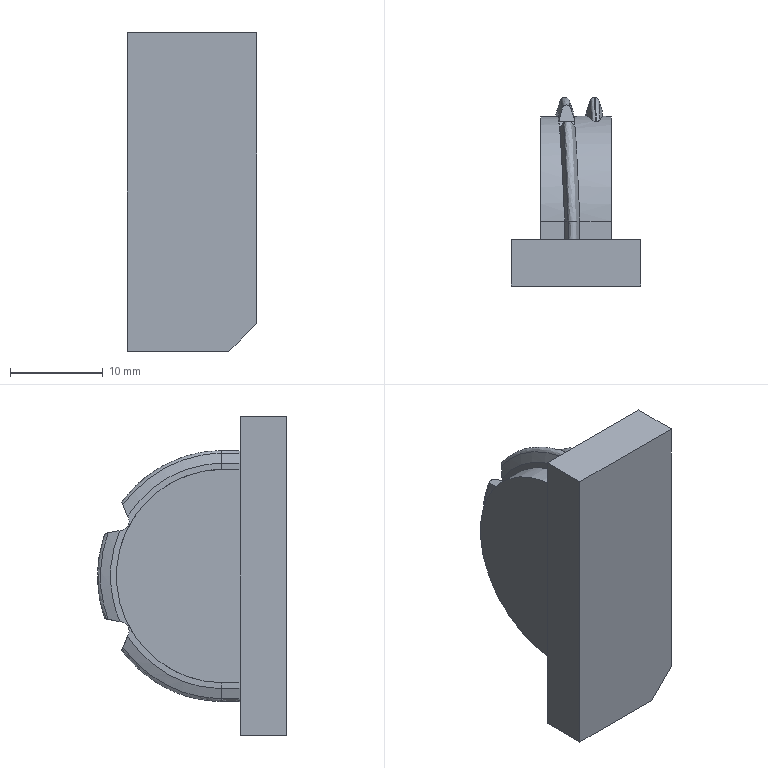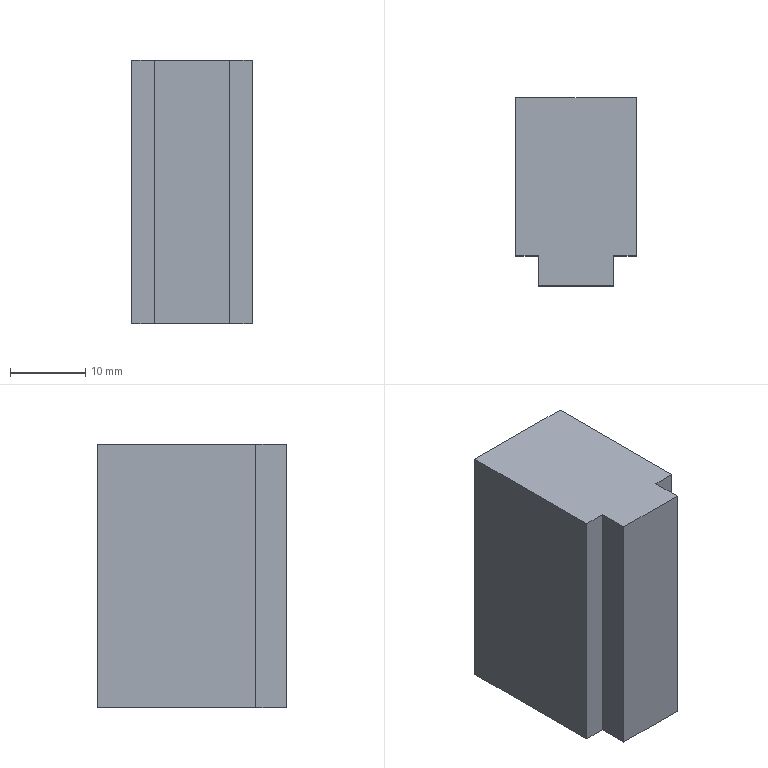CAM job | NX | 3-axis milling | part box 13.933 x 20.347 x 34.335 mm | stock box 16 x 25 x 35 mm
Tools:
number,name,description,diameter,corner_radius,flute_length,length,flutes
0,D4,Milling Tool-5 Parameters,4.0,0.0,50.0,75.0,2
0,D1.5,Milling Tool-5 Parameters,1.5,0.0,50.0,75.0,2
0,B1,Milling Tool-Ball Mill,1.0,0.5,50.0,75.0,2
Operations:
program,operation,operation_type,tool,method,geometry_group,spindle_rpm,surface_speed,feed_per_tooth,feed_cut,feed_plunge,cut_length_mm,path_length_mm,cut_time_min,machine_time_min
NC_PROGRAM,CAVITY_MILL,CavityMilling,D4,METHOD,WORKPIECE,8000.0,282.0,0.4178,2200.0,50.0,20671.34,21392.703,9.536,9.69
NC_PROGRAM,PLANAR_MILL,PlanarMilling,D4,METHOD,MCS_MILL,8000.0,282.0,0.4178,2200.0,50.0,2996.712,3128.614,1.388,1.41
NC_PROGRAM,CAVITY_MILL_COPY_1,CavityMilling,D4,METHOD,WORKPIECE,2992.0,282.0,0.4178,2500.0,50.0,240.951,277.541,0.098,0.1016
NC_PROGRAM,PLANAR_MILL_COPY,PlanarMilling,D4,METHOD,MCS_MILL,8000.0,100.0,0.0375,600.0,50.0,114.493,161.083,0.1945,0.1991
NC_PROGRAM,ZLEVEL_PROFILE,ZLevelMilling,D4,METHOD,WORKPIECE,8000.0,100.0,0.0375,600.0,50.0,477.872,542.535,0.834,0.8404
NC_PROGRAM,CAVITY_MILL_COPY,CavityMilling,D1.5,METHOD,WORKPIECE,2992.0,282.0,0.4178,2500.0,50.0,5174.195,7674.307,2.655,3.09
NC_PROGRAM,ZLEVEL_PROFILE_1,ZLevelMilling,B1,METHOD,WORKPIECE,3000.0,282.0,0.4167,2500.0,80.0,5273.925,5706.429,2.143,2.194
NC_PROGRAM,ZLEVEL_PROFILE_1_COPY,ZLevelMilling,B1,METHOD,WORKPIECE,3000.0,282.0,0.4167,2500.0,80.0,3462.586,3599.555,1.386,1.404
NC_PROGRAM,CONTOUR_AREA,SurfaceContour,B1,METHOD,WORKPIECE,3000.0,282.0,0.4167,2500.0,500.0,3515.219,3528.15,1.409,1.411
NC_PROGRAM,ZLEVEL_PROFILE_1_COPY_COPY,ZLevelMilling,B1,METHOD,MCS_MILL,3000.0,282.0,0.4167,2500.0,80.0,2863.422,2983.253,1.146,1.158
NC_PROGRAM,CONTOUR_AREA_COPY,SurfaceContour,B1,METHOD,MCS_MILL,3000.0,282.0,0.4167,2500.0,500.0,7534.29,7681.47,3.052,3.072
NC_PROGRAM,FIXED_CONTOUR,SurfaceContour,D1.5,METHOD,MCS_MILL,3000.0,282.0,0.4167,2500.0,500.0,15.131,23.927,0.0093,0.0101